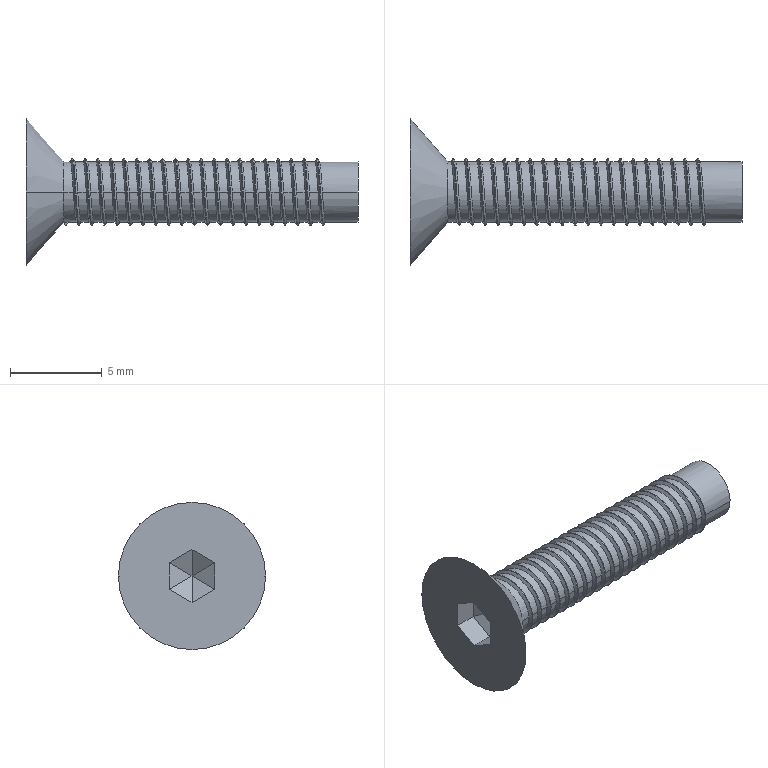Part | SolidWorks | features BlendCut 1, ICE 1, Revolution 1, SweepThread 1 | 1 solid | 63 faces | box 18.05 x 8 x 8 mm | volume 188.407 mm3 | cylinder 42 | plane 16 | spline 3 | cone 2 | commonest cylinder face diameters 3.3 x42